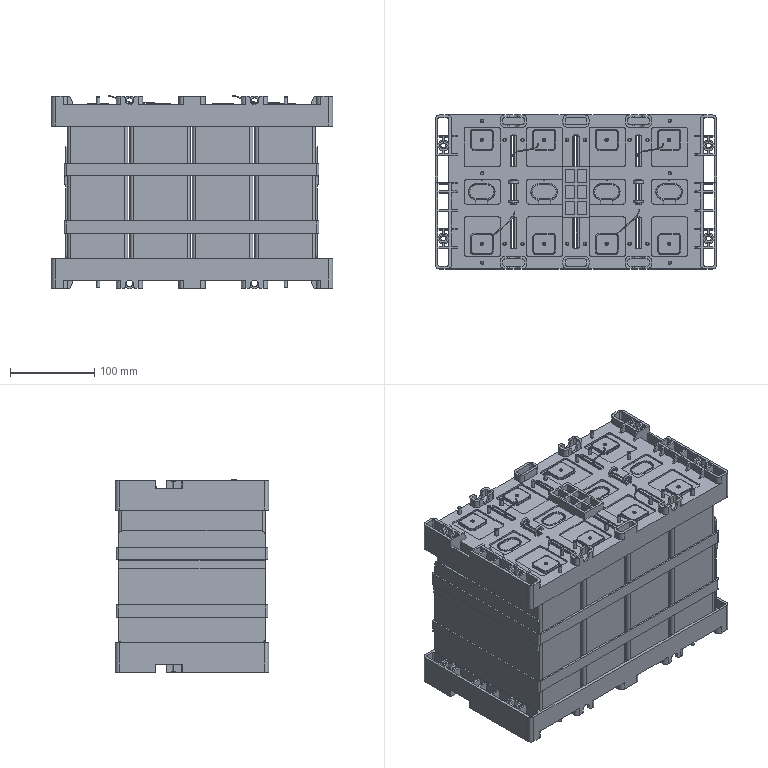Part | NX | features BREP 4 | 15 solids | 2676 faces | box 333 x 182 x 228.75 mm | volume 10791540 mm3 | plane 1740 | cylinder 784 | cone 120 | spline 24 | torus 8 | commonest cylinder face diameters 4 x216 6 x216 10 x100 2 x48 8 x32 4.22 x24